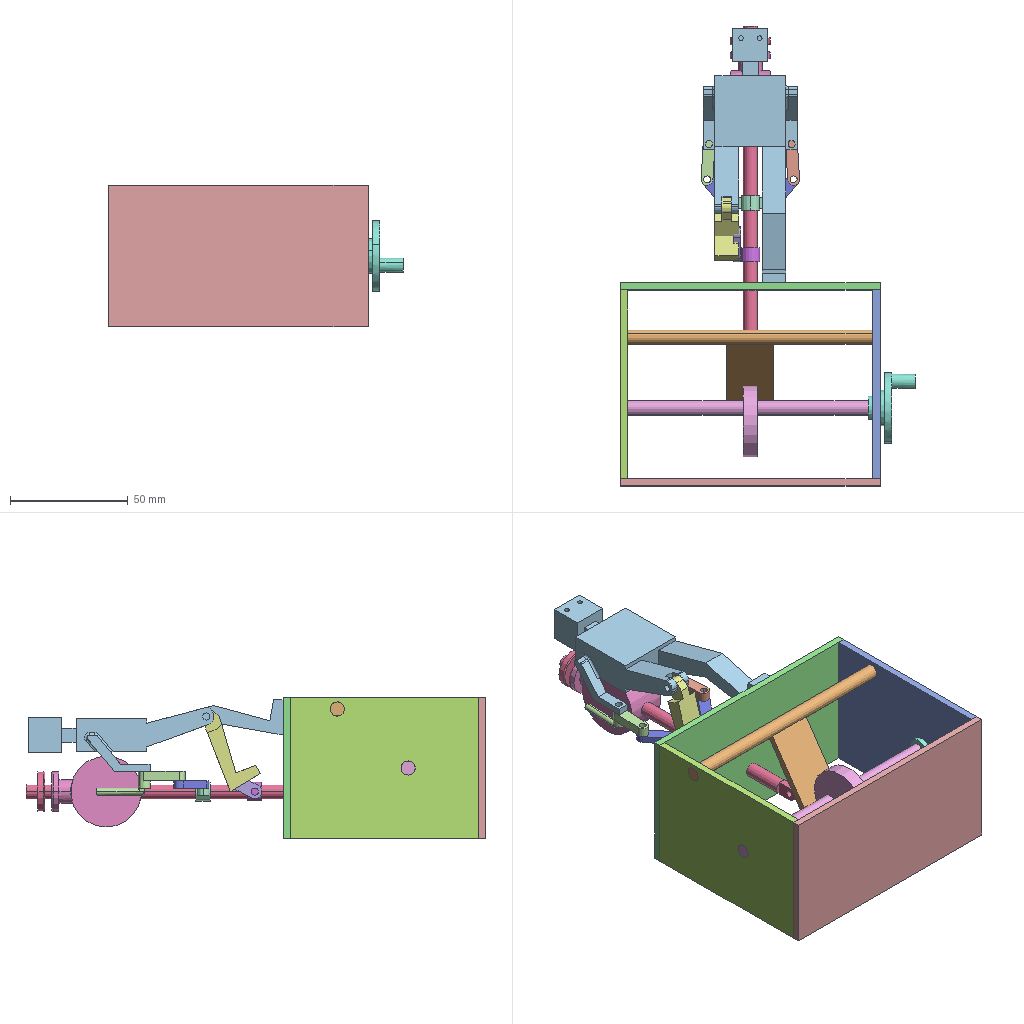Assembly | SolidWorks | 14 different items | 19 placed | box 125 x 195 x 60 mm
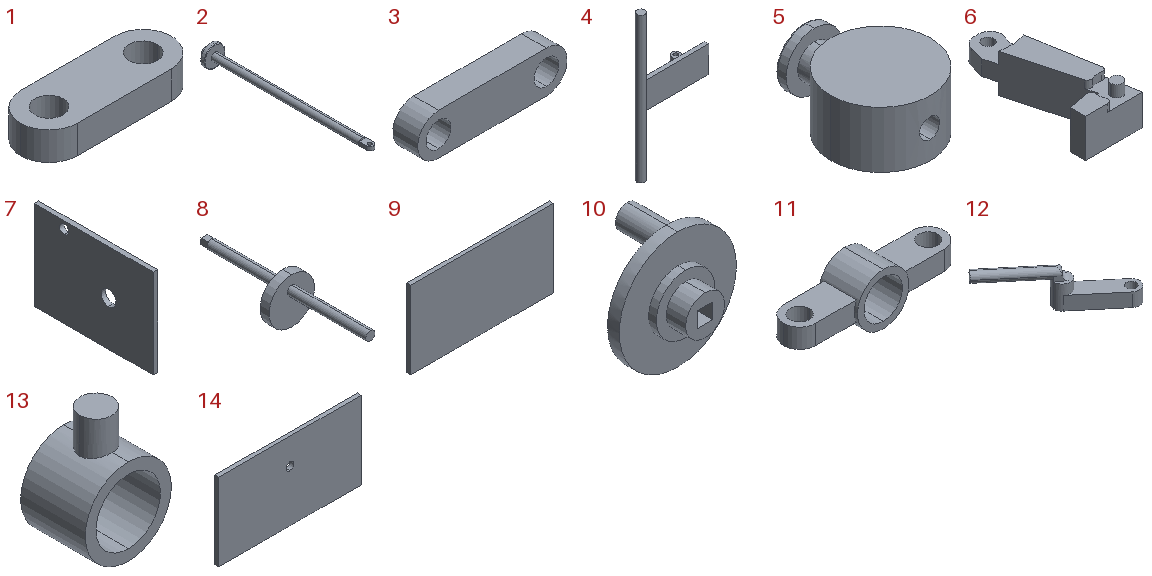Parts list (item | quantity | size | volume | features):
1 | x2 | 16 x 6 x 3 mm | 222.412 mm3 | features Extrusion 1
2 | x1 | 17 x 139 x 17 mm | 4398 mm3 | features ICE 2, Extrusion 1, Fillet 1
3 | x2 | 18 x 3 x 5 mm | 211.493 mm3 | features Extrusion 1
4 | x1 | 53 x 12.5 x 110 mm | 6049 mm3 | features ICE 2, Extrusion 1
5 | x1 | 30 x 38 x 17 mm | 12032 mm3 | features ICE 3, Extrusion 1, Fillet 1
6 | x2 | 15 x 35.544 x 11 mm | 2110 mm3 | features ICE 14, Fillet 5, MirrorPattern 2, Extrusion 1
7 | x2 | 3 x 80 x 60 mm | 14080 mm3 | features Extrusion 1, ICE 1
8 | x1 | 30 x 110 x 30 mm | 7120 mm3 | features ICE 2, Extrusion 1
9 | x1 | 110 x 3 x 60 mm | 19800 mm3 | features Extrusion 1
10 | x1 | 30 x 20 x 30 mm | 3069 mm3 | features ICE 4, Extrusion 1
11 | x1 | 25 x 6 x 8 mm | 331.315 mm3 | features Extrusion 1, ICE 1
12 | x2 | 30.276 x 26.147 x 10.13 mm | 535.495 mm3 | features ICE 3, Extrusion 1, Fillet 1, MirrorPattern 1
13 | x1 | 8 x 6 x 11 mm | 153.659 mm3 | features Extrusion 1, ICE 1
14 | x1 | 110 x 3 x 60 mm | 19715 mm3 | features Extrusion 1
Mates (type | each side: item.copy, entity, surface, feature):
Coincident | 9.1 plane | assembly plane | 3 times
Coincident | 9.1 face plane Boss-Extrude1 | 7.1 face plane Boss-Extrude1 | 3 times
Coincident | 9.1 face plane Boss-Extrude1 | 7.2 face plane Boss-Extrude1 | 3 times
Concentric | 7.2 face cylinder Boss-Extrude1 | 8.1 face cylinder Boss-Extrude2
Coincident | 7.2 face plane Boss-Extrude1 | 8.1 face plane Boss-Extrude2
Concentric | 7.1 face cylinder Cut-Extrude1 | 10.1 face cylinder Boss-Extrude3
Coincident | 8.1 face plane Cut-Extrude1 | 10.1 face plane Boss-Extrude4
Coincident | 8.1 face plane Boss-Extrude2 | 10.1 face plane Boss-Extrude3
Concentric | 7.2 face cylinder Boss-Extrude1 | 4.1 face cylinder Boss-Extrude1
Coincident | 7.2 face plane Boss-Extrude1 | 4.1 face plane Boss-Extrude1
Tangent | 8.1 face cylinder Boss-Extrude1 | 4.1 face plane Boss-Extrude2
Coincident | 4.1 face plane Boss-Extrude3 | 1.1 face plane Boss-Extrude1
Concentric | 4.1 face cylinder Boss-Extrude3 | 1.1 face cylinder Boss-Extrude1
Coincident | 7.1 face plane Boss-Extrude1 | 14.1 face plane Boss-Extrude1 | 2 times
Coincident | 7.2 face plane Boss-Extrude1 | 14.1 face plane Boss-Extrude1
Concentric | 14.1 face cylinder Boss-Extrude1 | 2.1 face cylinder Boss-Extrude1
Coincident | 1.1 face plane Boss-Extrude1 | 2.1 face plane Boss-Extrude2
Concentric | 1.1 face cylinder Boss-Extrude1 | 2.1 face cylinder Boss-Extrude2
Coincident | 14.1 face plane Boss-Extrude1 | 6.1 face plane Boss-Extrude1
Coincident | 6.1 face plane Cut-Extrude3 | 6.2 face plane Cut-Extrude8
Concentric | 6.1 face cylinder Cut-Extrude2 | 6.2 face cylinder Cut-Extrude6
Coincident | 6.1 plane | assembly plane
Concentric | 2.1 face cylinder Boss-Extrude1 | 13.1 face cylinder Boss-Extrude1
DistanceDim | 13.1 face plane Boss-Extrude1 | 2.1 face plane Boss-Extrude1
Concentric | 13.1 face cylinder Boss-Extrude2 | 1.2 face cylinder Boss-Extrude1
Coincident | 13.1 face plane Boss-Extrude2 | 1.2 face plane Boss-Extrude1
Concentric | 6.2 face cylinder Boss-Extrude7 | 1.2 face cylinder Boss-Extrude1
DistanceDim | 6.1 face plane Boss-Extrude1 | 14.1 face plane Boss-Extrude1
Concentric | 2.1 face cylinder Boss-Extrude1 | 11.1 face cylinder Boss-Extrude1
DistanceDim | 11.1 face plane Boss-Extrude1 | 2.1 face plane Boss-Extrude1
Coincident | 6.1 face plane Boss-Extrude4 | 12.1 face plane Boss-Extrude1
Concentric | 6.1 face cylinder Cut-Extrude11 | 12.1 face cylinder Boss-Extrude1
Coincident | 11.1 face plane Boss-Extrude2 | 3.1 face plane Boss-Extrude1
Concentric | 11.1 face cylinder Boss-Extrude2 | 3.1 face cylinder Boss-Extrude1
Concentric | 12.1 face cylinder Boss-Extrude1 | 3.1 face cylinder Boss-Extrude1
Coincident | 11.1 face plane Boss-Extrude2 | 3.2 face plane Boss-Extrude1
Concentric | 11.1 face cylinder Boss-Extrude2 | 3.2 face cylinder Boss-Extrude1
Coincident | 6.1 face plane Mirror1 | 12.2 face plane Boss-Extrude1
Concentric | 3.2 face cylinder Boss-Extrude1 | 12.2 face cylinder Boss-Extrude1
Concentric | 6.1 face cylinder Cut-Extrude11 | 12.2 face cylinder Boss-Extrude1
Concentric | 2.1 face cylinder Boss-Extrude1 | 5.1 face cylinder Cut-Extrude1
Parallel | 14.1 face plane Boss-Extrude1 | 5.1 face plane Boss-Extrude1
DistanceDim | 5.1 plane | 14.1 face plane Boss-Extrude1